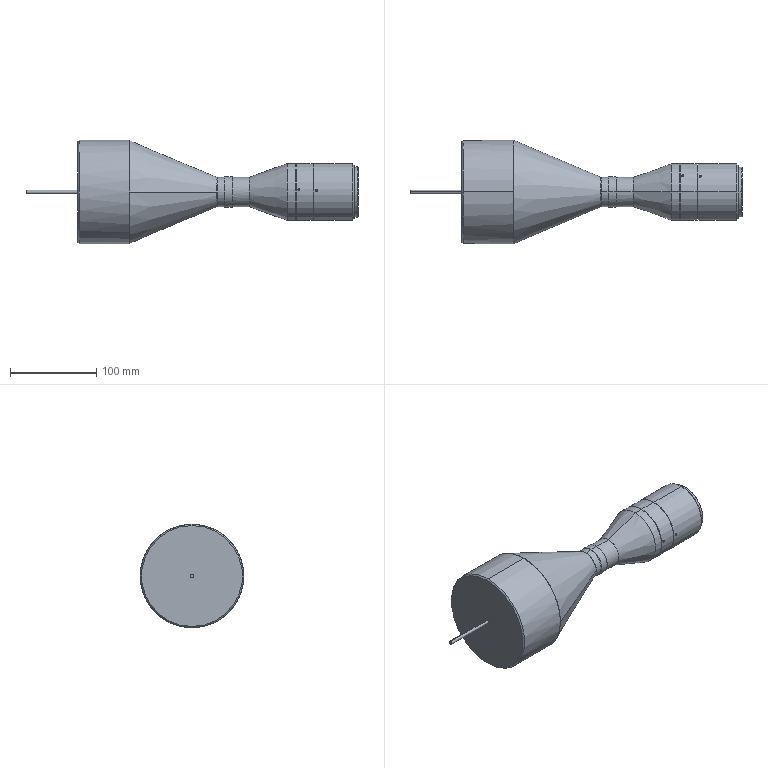Part | SolidWorks | features BaseBody 1, ICE 1 | 1 solid | 79 faces | box 384.7 x 120 x 120 mm | volume 1601205 mm3 | cylinder 36 | cone 28 | plane 9 | spline 6 | commonest cylinder face diameters 2.5 x12 66 x6 34 x4 59 x4 4 x2 35 x2